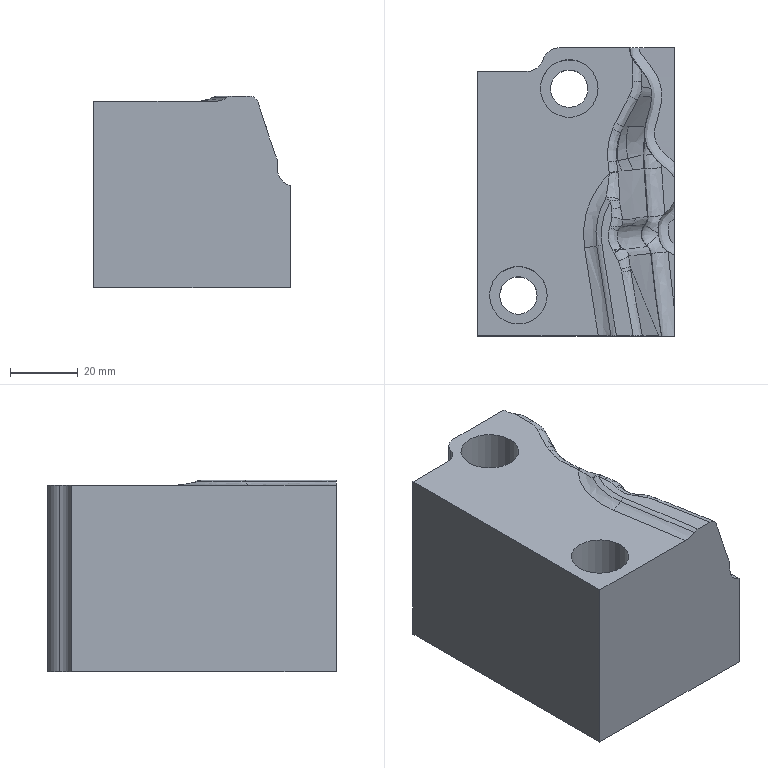Part | STEP file | 1 solid | 89 faces | box 58 x 85 x 56.501 mm | volume 217515 mm3 | spline 71 | plane 12 | cylinder 6 | commonest cylinder face diameters 10 x2 11 x2 17 x2